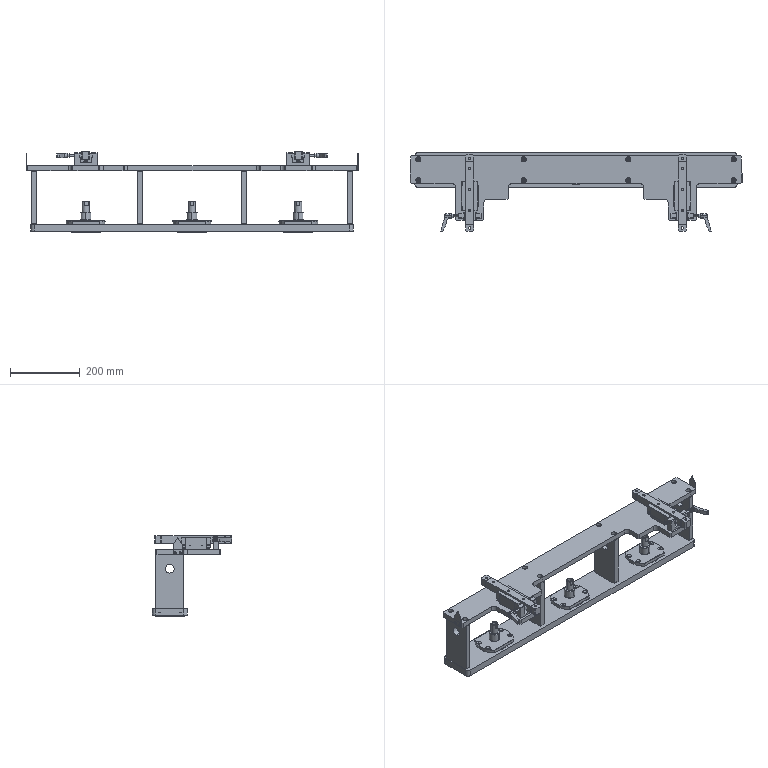Part | SolidWorks | features ReferencePattern 11, MirrorCompFeat 2, CompositeCurve 1, LocalLPattern 1 | 35 solids | 1148 faces | box 953 x 227 x 231.5 mm | volume 4552776 mm3 | plane 519 | cylinder 470 | cone 155 | torus 4 | commonest cylinder face diameters 5 x48 6 x46 6.6 x44 6.8 x40 9 x40 15 x32